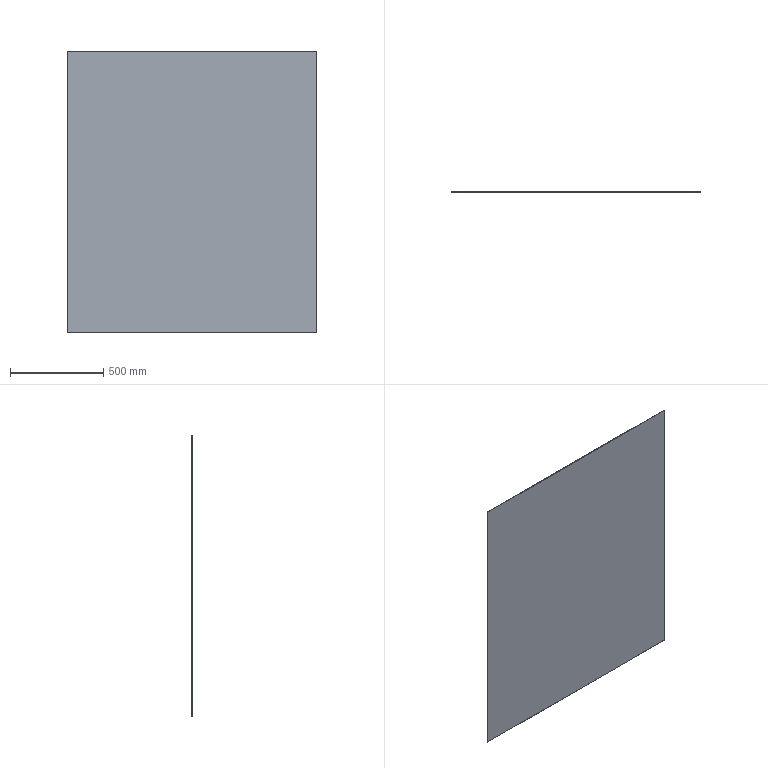Part | STEP file | PN_0011 Sealing plate | 1 solid | 6 faces | box 1340 x 3 x 1510 mm | volume 6070200 mm3 | plane 6
STEP:
#1=CARTESIAN_POINT('',(0.,0.,0.));
#2=DIRECTION('',(0.,0.,1.));
#3=DIRECTION('',(1.,0.,0.));
#4=AXIS2_PLACEMENT_3D('',#1,#2,#3);
#5=CARTESIAN_POINT('',(0.,0.,0.));
#6=VERTEX_POINT('',#5);
#7=CARTESIAN_POINT('',(0.,0.,1510.));
#8=VERTEX_POINT('',#7);
#9=CARTESIAN_POINT('',(0.,0.,0.));
#10=DIRECTION('',(0.,0.,1.));
#11=VECTOR('',#10,1.);
#12=LINE('',#9,#11);
#13=CARTESIAN_POINT('',(0.,3.,0.));
#14=DIRECTION('',(1.,0.,0.));
#15=DIRECTION('',(0.,0.,-1.));
#16=AXIS2_PLACEMENT_3D('',#13,#14,#15);
#17=PLANE('',#16);
#18=CARTESIAN_POINT('',(0.,-3.));
#19=DIRECTION('',(-1.,0.));
#20=VECTOR('',#19,1.);
#21=LINE('',#18,#20);
#22=(GEOMETRIC_REPRESENTATION_CONTEXT(2)PARAMETRIC_REPRESENTATION_CONTEXT()REPRESENTATION_CONTEXT('',''));
#23=DEFINITIONAL_REPRESENTATION('',(#21),#22);
#24=PCURVE('',#17,#23);
#25=CARTESIAN_POINT('',(0.,0.,1510.));
#26=DIRECTION('',(0.,1.,0.));
#27=DIRECTION('',(0.,0.,1.));
#28=AXIS2_PLACEMENT_3D('',#25,#26,#27);
#29=PLANE('',#28);
#30=CARTESIAN_POINT('',(-1510.,0.));
#31=DIRECTION('',(1.,0.));
#32=VECTOR('',#31,1.);
#33=LINE('',#30,#32);
#34=(GEOMETRIC_REPRESENTATION_CONTEXT(2)PARAMETRIC_REPRESENTATION_CONTEXT()REPRESENTATION_CONTEXT('',''));
#35=DEFINITIONAL_REPRESENTATION('',(#33),#34);
#36=PCURVE('',#29,#35);
#37=SURFACE_CURVE('',#12,(#24,#36),.PCURVE_S1.);
#38=EDGE_CURVE('',#6,#8,#37,.T.);
#39=ORIENTED_EDGE('',*,*,#38,.T.);
#40=CARTESIAN_POINT('',(0.,3.,1510.));
#41=VERTEX_POINT('',#40);
#42=CARTESIAN_POINT('',(0.,3.,1510.));
#43=DIRECTION('',(0.,-1.,0.));
#44=VECTOR('',#43,1.);
#45=LINE('',#42,#44);
#46=CARTESIAN_POINT('',(-1510.,0.));
#47=DIRECTION('',(0.,-1.));
#48=VECTOR('',#47,1.);
#49=LINE('',#46,#48);
#50=(GEOMETRIC_REPRESENTATION_CONTEXT(2)PARAMETRIC_REPRESENTATION_CONTEXT()REPRESENTATION_CONTEXT('',''));
#51=DEFINITIONAL_REPRESENTATION('',(#49),#50);
#52=PCURVE('',#17,#51);
#53=CARTESIAN_POINT('',(0.,3.,1510.));
#54=DIRECTION('',(0.,0.,-1.));
#55=DIRECTION('',(-1.,0.,0.));
#56=AXIS2_PLACEMENT_3D('',#53,#54,#55);
#57=PLANE('',#56);
#58=CARTESIAN_POINT('',(0.,0.));
#59=DIRECTION('',(0.,-1.));
#60=VECTOR('',#59,1.);
#61=LINE('',#58,#60);
#62=(GEOMETRIC_REPRESENTATION_CONTEXT(2)PARAMETRIC_REPRESENTATION_CONTEXT()REPRESENTATION_CONTEXT('',''));
#63=DEFINITIONAL_REPRESENTATION('',(#61),#62);
#64=PCURVE('',#57,#63);
#65=SURFACE_CURVE('',#45,(#52,#64),.PCURVE_S1.);
#66=EDGE_CURVE('',#41,#8,#65,.T.);
#67=ORIENTED_EDGE('',*,*,#66,.F.);
#68=CARTESIAN_POINT('',(0.,3.,0.));
#69=VERTEX_POINT('',#68);
#70=CARTESIAN_POINT('',(0.,3.,0.));
#71=DIRECTION('',(0.,0.,1.));
#72=VECTOR('',#71,1.);
#73=LINE('',#70,#72);
#74=CARTESIAN_POINT('',(0.,0.));
#75=DIRECTION('',(-1.,0.));
#76=VECTOR('',#75,1.);
#77=LINE('',#74,#76);
#78=(GEOMETRIC_REPRESENTATION_CONTEXT(2)PARAMETRIC_REPRESENTATION_CONTEXT()REPRESENTATION_CONTEXT('',''));
#79=DEFINITIONAL_REPRESENTATION('',(#77),#78);
#80=PCURVE('',#17,#79);
#81=CARTESIAN_POINT('',(0.,3.,1510.));
#82=DIRECTION('',(0.,1.,0.));
#83=DIRECTION('',(0.,0.,1.));
#84=AXIS2_PLACEMENT_3D('',#81,#82,#83);
#85=PLANE('',#84);
#86=CARTESIAN_POINT('',(-1510.,0.));
#87=DIRECTION('',(1.,0.));
#88=VECTOR('',#87,1.);
#89=LINE('',#86,#88);
#90=(GEOMETRIC_REPRESENTATION_CONTEXT(2)PARAMETRIC_REPRESENTATION_CONTEXT()REPRESENTATION_CONTEXT('',''));
#91=DEFINITIONAL_REPRESENTATION('',(#89),#90);
#92=PCURVE('',#85,#91);
#93=SURFACE_CURVE('',#73,(#80,#92),.PCURVE_S1.);
#94=EDGE_CURVE('',#69,#41,#93,.T.);
#95=ORIENTED_EDGE('',*,*,#94,.F.);
#96=CARTESIAN_POINT('',(0.,3.,0.));
#97=DIRECTION('',(0.,-1.,0.));
#98=VECTOR('',#97,1.);
#99=LINE('',#96,#98);
#100=CARTESIAN_POINT('',(0.,0.));
#101=DIRECTION('',(0.,-1.));
#102=VECTOR('',#101,1.);
#103=LINE('',#100,#102);
#104=(GEOMETRIC_REPRESENTATION_CONTEXT(2)PARAMETRIC_REPRESENTATION_CONTEXT()REPRESENTATION_CONTEXT('',''));
#105=DEFINITIONAL_REPRESENTATION('',(#103),#104);
#106=PCURVE('',#17,#105);
#107=CARTESIAN_POINT('',(0.,3.,0.));
#108=DIRECTION('',(0.,0.,1.));
#109=DIRECTION('',(1.,0.,0.));
#110=AXIS2_PLACEMENT_3D('',#107,#108,#109);
#111=PLANE('',#110);
#112=CARTESIAN_POINT('',(0.,0.));
#113=DIRECTION('',(0.,-1.));
#114=VECTOR('',#113,1.);
#115=LINE('',#112,#114);
#116=(GEOMETRIC_REPRESENTATION_CONTEXT(2)PARAMETRIC_REPRESENTATION_CONTEXT()REPRESENTATION_CONTEXT('',''));
#117=DEFINITIONAL_REPRESENTATION('',(#115),#116);
#118=PCURVE('',#111,#117);
#119=SURFACE_CURVE('',#99,(#106,#118),.PCURVE_S1.);
#120=EDGE_CURVE('',#69,#6,#119,.T.);
#121=ORIENTED_EDGE('',*,*,#120,.T.);
#122=EDGE_LOOP('',(#39,#67,#95,#121));
#123=FACE_BOUND('',#122,.T.);
#124=ADVANCED_FACE('',(#123),#17,.F.);
#125=CARTESIAN_POINT('',(1340.,0.,1510.));
#126=VERTEX_POINT('',#125);
#127=CARTESIAN_POINT('',(0.,0.,1510.));
#128=DIRECTION('',(1.,0.,0.));
#129=VECTOR('',#128,1.);
#130=LINE('',#127,#129);
#131=CARTESIAN_POINT('',(0.,-3.));
#132=DIRECTION('',(-1.,0.));
#133=VECTOR('',#132,1.);
#134=LINE('',#131,#133);
#135=(GEOMETRIC_REPRESENTATION_CONTEXT(2)PARAMETRIC_REPRESENTATION_CONTEXT()REPRESENTATION_CONTEXT('',''));
#136=DEFINITIONAL_REPRESENTATION('',(#134),#135);
#137=PCURVE('',#57,#136);
#138=CARTESIAN_POINT('',(0.,0.));
#139=DIRECTION('',(0.,1.));
#140=VECTOR('',#139,1.);
#141=LINE('',#138,#140);
#142=(GEOMETRIC_REPRESENTATION_CONTEXT(2)PARAMETRIC_REPRESENTATION_CONTEXT()REPRESENTATION_CONTEXT('',''));
#143=DEFINITIONAL_REPRESENTATION('',(#141),#142);
#144=PCURVE('',#29,#143);
#145=SURFACE_CURVE('',#130,(#137,#144),.PCURVE_S1.);
#146=EDGE_CURVE('',#8,#126,#145,.T.);
#147=ORIENTED_EDGE('',*,*,#146,.T.);
#148=CARTESIAN_POINT('',(1340.,3.,1510.));
#149=VERTEX_POINT('',#148);
#150=CARTESIAN_POINT('',(1340.,3.,1510.));
#151=DIRECTION('',(0.,-1.,0.));
#152=VECTOR('',#151,1.);
#153=LINE('',#150,#152);
#154=CARTESIAN_POINT('',(-1340.,0.));
#155=DIRECTION('',(0.,-1.));
#156=VECTOR('',#155,1.);
#157=LINE('',#154,#156);
#158=(GEOMETRIC_REPRESENTATION_CONTEXT(2)PARAMETRIC_REPRESENTATION_CONTEXT()REPRESENTATION_CONTEXT('',''));
#159=DEFINITIONAL_REPRESENTATION('',(#157),#158);
#160=PCURVE('',#57,#159);
#161=CARTESIAN_POINT('',(1340.,3.,0.));
#162=DIRECTION('',(-1.,0.,0.));
#163=DIRECTION('',(0.,0.,1.));
#164=AXIS2_PLACEMENT_3D('',#161,#162,#163);
#165=PLANE('',#164);
#166=CARTESIAN_POINT('',(1510.,0.));
#167=DIRECTION('',(0.,-1.));
#168=VECTOR('',#167,1.);
#169=LINE('',#166,#168);
#170=(GEOMETRIC_REPRESENTATION_CONTEXT(2)PARAMETRIC_REPRESENTATION_CONTEXT()REPRESENTATION_CONTEXT('',''));
#171=DEFINITIONAL_REPRESENTATION('',(#169),#170);
#172=PCURVE('',#165,#171);
#173=SURFACE_CURVE('',#153,(#160,#172),.PCURVE_S1.);
#174=EDGE_CURVE('',#149,#126,#173,.T.);
#175=ORIENTED_EDGE('',*,*,#174,.F.);
#176=CARTESIAN_POINT('',(0.,3.,1510.));
#177=DIRECTION('',(1.,0.,0.));
#178=VECTOR('',#177,1.);
#179=LINE('',#176,#178);
#180=CARTESIAN_POINT('',(0.,0.));
#181=DIRECTION('',(-1.,0.));
#182=VECTOR('',#181,1.);
#183=LINE('',#180,#182);
#184=(GEOMETRIC_REPRESENTATION_CONTEXT(2)PARAMETRIC_REPRESENTATION_CONTEXT()REPRESENTATION_CONTEXT('',''));
#185=DEFINITIONAL_REPRESENTATION('',(#183),#184);
#186=PCURVE('',#57,#185);
#187=CARTESIAN_POINT('',(0.,0.));
#188=DIRECTION('',(0.,1.));
#189=VECTOR('',#188,1.);
#190=LINE('',#187,#189);
#191=(GEOMETRIC_REPRESENTATION_CONTEXT(2)PARAMETRIC_REPRESENTATION_CONTEXT()REPRESENTATION_CONTEXT('',''));
#192=DEFINITIONAL_REPRESENTATION('',(#190),#191);
#193=PCURVE('',#85,#192);
#194=SURFACE_CURVE('',#179,(#186,#193),.PCURVE_S1.);
#195=EDGE_CURVE('',#41,#149,#194,.T.);
#196=ORIENTED_EDGE('',*,*,#195,.F.);
#197=ORIENTED_EDGE('',*,*,#66,.T.);
#198=EDGE_LOOP('',(#147,#175,#196,#197));
#199=FACE_BOUND('',#198,.T.);
#200=ADVANCED_FACE('',(#199),#57,.F.);
#201=CARTESIAN_POINT('',(1340.,0.,0.));
#202=VERTEX_POINT('',#201);
#203=CARTESIAN_POINT('',(1340.,0.,0.));
#204=DIRECTION('',(0.,0.,-1.));
#205=VECTOR('',#204,1.);
#206=LINE('',#203,#205);
#207=CARTESIAN_POINT('',(0.,-3.));
#208=DIRECTION('',(-1.,0.));
#209=VECTOR('',#208,1.);
#210=LINE('',#207,#209);
#211=(GEOMETRIC_REPRESENTATION_CONTEXT(2)PARAMETRIC_REPRESENTATION_CONTEXT()REPRESENTATION_CONTEXT('',''));
#212=DEFINITIONAL_REPRESENTATION('',(#210),#211);
#213=PCURVE('',#165,#212);
#214=CARTESIAN_POINT('',(-1510.,1340.));
#215=DIRECTION('',(-1.,0.));
#216=VECTOR('',#215,1.);
#217=LINE('',#214,#216);
#218=(GEOMETRIC_REPRESENTATION_CONTEXT(2)PARAMETRIC_REPRESENTATION_CONTEXT()REPRESENTATION_CONTEXT('',''));
#219=DEFINITIONAL_REPRESENTATION('',(#217),#218);
#220=PCURVE('',#29,#219);
#221=SURFACE_CURVE('',#206,(#213,#220),.PCURVE_S1.);
#222=EDGE_CURVE('',#126,#202,#221,.T.);
#223=ORIENTED_EDGE('',*,*,#222,.T.);
#224=CARTESIAN_POINT('',(1340.,3.,0.));
#225=VERTEX_POINT('',#224);
#226=CARTESIAN_POINT('',(1340.,3.,0.));
#227=DIRECTION('',(0.,-1.,0.));
#228=VECTOR('',#227,1.);
#229=LINE('',#226,#228);
#230=CARTESIAN_POINT('',(0.,0.));
#231=DIRECTION('',(0.,-1.));
#232=VECTOR('',#231,1.);
#233=LINE('',#230,#232);
#234=(GEOMETRIC_REPRESENTATION_CONTEXT(2)PARAMETRIC_REPRESENTATION_CONTEXT()REPRESENTATION_CONTEXT('',''));
#235=DEFINITIONAL_REPRESENTATION('',(#233),#234);
#236=PCURVE('',#165,#235);
#237=CARTESIAN_POINT('',(1340.,0.));
#238=DIRECTION('',(0.,-1.));
#239=VECTOR('',#238,1.);
#240=LINE('',#237,#239);
#241=(GEOMETRIC_REPRESENTATION_CONTEXT(2)PARAMETRIC_REPRESENTATION_CONTEXT()REPRESENTATION_CONTEXT('',''));
#242=DEFINITIONAL_REPRESENTATION('',(#240),#241);
#243=PCURVE('',#111,#242);
#244=SURFACE_CURVE('',#229,(#236,#243),.PCURVE_S1.);
#245=EDGE_CURVE('',#225,#202,#244,.T.);
#246=ORIENTED_EDGE('',*,*,#245,.F.);
#247=CARTESIAN_POINT('',(1340.,3.,0.));
#248=DIRECTION('',(0.,0.,-1.));
#249=VECTOR('',#248,1.);
#250=LINE('',#247,#249);
#251=CARTESIAN_POINT('',(0.,0.));
#252=DIRECTION('',(-1.,0.));
#253=VECTOR('',#252,1.);
#254=LINE('',#251,#253);
#255=(GEOMETRIC_REPRESENTATION_CONTEXT(2)PARAMETRIC_REPRESENTATION_CONTEXT()REPRESENTATION_CONTEXT('',''));
#256=DEFINITIONAL_REPRESENTATION('',(#254),#255);
#257=PCURVE('',#165,#256);
#258=CARTESIAN_POINT('',(-1510.,1340.));
#259=DIRECTION('',(-1.,0.));
#260=VECTOR('',#259,1.);
#261=LINE('',#258,#260);
#262=(GEOMETRIC_REPRESENTATION_CONTEXT(2)PARAMETRIC_REPRESENTATION_CONTEXT()REPRESENTATION_CONTEXT('',''));
#263=DEFINITIONAL_REPRESENTATION('',(#261),#262);
#264=PCURVE('',#85,#263);
#265=SURFACE_CURVE('',#250,(#257,#264),.PCURVE_S1.);
#266=EDGE_CURVE('',#149,#225,#265,.T.);
#267=ORIENTED_EDGE('',*,*,#266,.F.);
#268=ORIENTED_EDGE('',*,*,#174,.T.);
#269=EDGE_LOOP('',(#223,#246,#267,#268));
#270=FACE_BOUND('',#269,.T.);
#271=ADVANCED_FACE('',(#270),#165,.F.);
#272=CARTESIAN_POINT('',(0.,0.,0.));
#273=DIRECTION('',(-1.,0.,0.));
#274=VECTOR('',#273,1.);
#275=LINE('',#272,#274);
#276=CARTESIAN_POINT('',(0.,-3.));
#277=DIRECTION('',(-1.,0.));
#278=VECTOR('',#277,1.);
#279=LINE('',#276,#278);
#280=(GEOMETRIC_REPRESENTATION_CONTEXT(2)PARAMETRIC_REPRESENTATION_CONTEXT()REPRESENTATION_CONTEXT('',''));
#281=DEFINITIONAL_REPRESENTATION('',(#279),#280);
#282=PCURVE('',#111,#281);
#283=CARTESIAN_POINT('',(-1510.,0.));
#284=DIRECTION('',(0.,-1.));
#285=VECTOR('',#284,1.);
#286=LINE('',#283,#285);
#287=(GEOMETRIC_REPRESENTATION_CONTEXT(2)PARAMETRIC_REPRESENTATION_CONTEXT()REPRESENTATION_CONTEXT('',''));
#288=DEFINITIONAL_REPRESENTATION('',(#286),#287);
#289=PCURVE('',#29,#288);
#290=SURFACE_CURVE('',#275,(#282,#289),.PCURVE_S1.);
#291=EDGE_CURVE('',#202,#6,#290,.T.);
#292=ORIENTED_EDGE('',*,*,#291,.T.);
#293=ORIENTED_EDGE('',*,*,#120,.F.);
#294=CARTESIAN_POINT('',(0.,3.,0.));
#295=DIRECTION('',(-1.,0.,0.));
#296=VECTOR('',#295,1.);
#297=LINE('',#294,#296);
#298=CARTESIAN_POINT('',(0.,0.));
#299=DIRECTION('',(-1.,0.));
#300=VECTOR('',#299,1.);
#301=LINE('',#298,#300);
#302=(GEOMETRIC_REPRESENTATION_CONTEXT(2)PARAMETRIC_REPRESENTATION_CONTEXT()REPRESENTATION_CONTEXT('',''));
#303=DEFINITIONAL_REPRESENTATION('',(#301),#302);
#304=PCURVE('',#111,#303);
#305=CARTESIAN_POINT('',(-1510.,0.));
#306=DIRECTION('',(0.,-1.));
#307=VECTOR('',#306,1.);
#308=LINE('',#305,#307);
#309=(GEOMETRIC_REPRESENTATION_CONTEXT(2)PARAMETRIC_REPRESENTATION_CONTEXT()REPRESENTATION_CONTEXT('',''));
#310=DEFINITIONAL_REPRESENTATION('',(#308),#309);
#311=PCURVE('',#85,#310);
#312=SURFACE_CURVE('',#297,(#304,#311),.PCURVE_S1.);
#313=EDGE_CURVE('',#225,#69,#312,.T.);
#314=ORIENTED_EDGE('',*,*,#313,.F.);
#315=ORIENTED_EDGE('',*,*,#245,.T.);
#316=EDGE_LOOP('',(#292,#293,#314,#315));
#317=FACE_BOUND('',#316,.T.);
#318=ADVANCED_FACE('',(#317),#111,.F.);
#319=ORIENTED_EDGE('',*,*,#94,.T.);
#320=ORIENTED_EDGE('',*,*,#195,.T.);
#321=ORIENTED_EDGE('',*,*,#266,.T.);
#322=ORIENTED_EDGE('',*,*,#313,.T.);
#323=EDGE_LOOP('',(#319,#320,#321,#322));
#324=FACE_BOUND('',#323,.T.);
#325=ADVANCED_FACE('',(#324),#85,.T.);
#326=ORIENTED_EDGE('',*,*,#38,.F.);
#327=ORIENTED_EDGE('',*,*,#291,.F.);
#328=ORIENTED_EDGE('',*,*,#222,.F.);
#329=ORIENTED_EDGE('',*,*,#146,.F.);
#330=EDGE_LOOP('',(#326,#327,#328,#329));
#331=FACE_BOUND('',#330,.T.);
#332=ADVANCED_FACE('',(#331),#29,.F.);
#333=CLOSED_SHELL('',(#124,#200,#271,#318,#325,#332));
#334=MANIFOLD_SOLID_BREP('',#333);
#335=(LENGTH_UNIT()NAMED_UNIT(*)SI_UNIT(.MILLI.,.METRE.));
#336=UNCERTAINTY_MEASURE_WITH_UNIT(LENGTH_MEASURE(0.0000001),#335,'','');
#337=(NAMED_UNIT(*)PLANE_ANGLE_UNIT()SI_UNIT($,.RADIAN.));
#338=(NAMED_UNIT(*)SI_UNIT($,.STERADIAN.)SOLID_ANGLE_UNIT());
#339=(GEOMETRIC_REPRESENTATION_CONTEXT(3)GLOBAL_UNCERTAINTY_ASSIGNED_CONTEXT((#336))GLOBAL_UNIT_ASSIGNED_CONTEXT((#335,#337,#338))REPRESENTATION_CONTEXT('',''));
#340=ADVANCED_BREP_SHAPE_REPRESENTATION('',(#4,#334),#339);